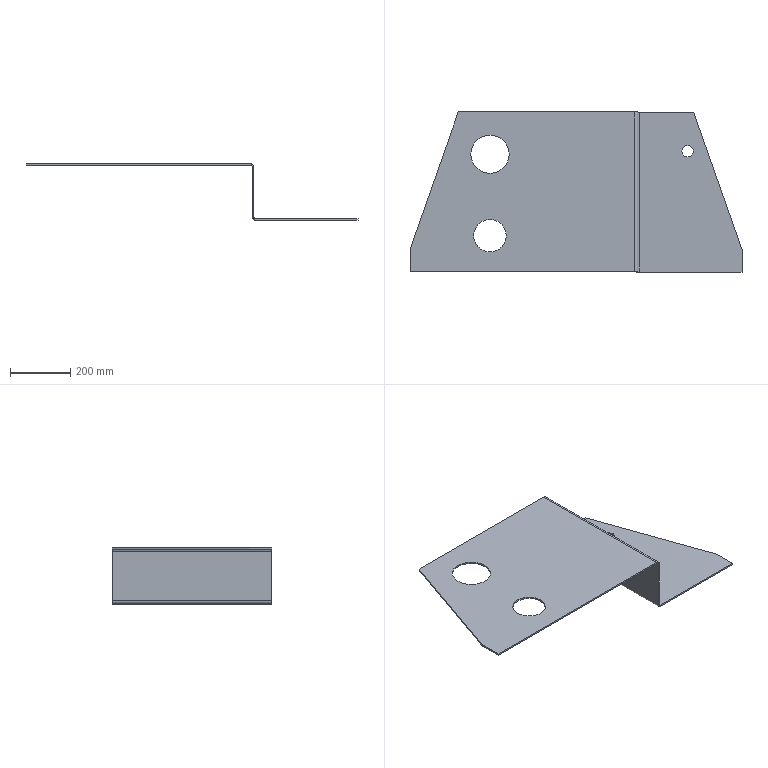Part | SolidWorks | features Cut 2, EdgeFlange 2, ICE 2, FlatPattern 1, SMBaseFlange 1, SheetMetal 1, UnFold 1 | 1 solid | 30 faces | box 1100 x 530 x 187 mm | volume 2899151 mm3 | plane 20 | cylinder 10 | commonest cylinder face diameters 12 x2 22 x2 38 x2 108 x2 127 x2
STEP:
#1=CARTESIAN_POINT('',(389.,400.,-182.));
#2=VERTEX_POINT('',#1);
#3=CARTESIAN_POINT('',(351.,400.,-182.));
#4=VERTEX_POINT('',#3);
#5=CARTESIAN_POINT('',(370.,400.,-182.));
#6=DIRECTION('',(0.,0.,-1.));
#7=DIRECTION('',(-1.,0.,0.));
#8=AXIS2_PLACEMENT_3D('',#5,#6,#7);
#9=CIRCLE('',#8,19.);
#10=EDGE_CURVE('',#2,#4,#9,.T.);
#11=ORIENTED_EDGE('',*,*,#10,.F.);
#12=CARTESIAN_POINT('',(389.,400.,-187.));
#13=VERTEX_POINT('',#12);
#14=CARTESIAN_POINT('',(389.,400.,-177.));
#15=DIRECTION('',(0.,0.,-1.));
#16=VECTOR('',#15,1000.);
#17=LINE('',#14,#16);
#18=EDGE_CURVE('',#2,#13,#17,.T.);
#19=ORIENTED_EDGE('',*,*,#18,.T.);
#20=CARTESIAN_POINT('',(351.,400.,-187.));
#21=VERTEX_POINT('',#20);
#22=CARTESIAN_POINT('',(370.,400.,-187.));
#23=DIRECTION('',(0.,0.,-1.));
#24=DIRECTION('',(-1.,0.,0.));
#25=AXIS2_PLACEMENT_3D('',#22,#23,#24);
#26=CIRCLE('',#25,19.);
#27=EDGE_CURVE('',#13,#21,#26,.T.);
#28=ORIENTED_EDGE('',*,*,#27,.T.);
#29=CARTESIAN_POINT('',(351.,400.,-177.));
#30=DIRECTION('',(0.,0.,-1.));
#31=VECTOR('',#30,1000.);
#32=LINE('',#29,#31);
#33=EDGE_CURVE('',#4,#21,#32,.T.);
#34=ORIENTED_EDGE('',*,*,#33,.F.);
#35=EDGE_LOOP('',(#11,#19,#28,#34));
#36=FACE_OUTER_BOUND('',#35,.T.);
#37=CARTESIAN_POINT('',(370.,400.,-177.));
#38=DIRECTION('',(0.,0.,-1.));
#39=DIRECTION('',(-1.,0.,0.));
#40=AXIS2_PLACEMENT_3D('',#37,#38,#39);
#41=CYLINDRICAL_SURFACE('',#40,19.);
#42=ADVANCED_FACE('',(#36),#41,.F.);
#43=CARTESIAN_POINT('',(-231.,120.,0.));
#44=VERTEX_POINT('',#43);
#45=CARTESIAN_POINT('',(-339.,120.,0.));
#46=VERTEX_POINT('',#45);
#47=CARTESIAN_POINT('',(-285.,120.,0.));
#48=DIRECTION('',(0.,0.,-1.));
#49=DIRECTION('',(-1.,0.,0.));
#50=AXIS2_PLACEMENT_3D('',#47,#48,#49);
#51=CIRCLE('',#50,54.);
#52=EDGE_CURVE('',#44,#46,#51,.T.);
#53=ORIENTED_EDGE('',*,*,#52,.F.);
#54=CARTESIAN_POINT('',(-231.,120.,-5.));
#55=VERTEX_POINT('',#54);
#56=CARTESIAN_POINT('',(-231.,120.,265.));
#57=DIRECTION('',(0.,0.,-1.));
#58=VECTOR('',#57,1000.);
#59=LINE('',#56,#58);
#60=EDGE_CURVE('',#44,#55,#59,.T.);
#61=ORIENTED_EDGE('',*,*,#60,.T.);
#62=CARTESIAN_POINT('',(-339.,120.,-5.));
#63=VERTEX_POINT('',#62);
#64=CARTESIAN_POINT('',(-285.,120.,-5.));
#65=DIRECTION('',(0.,0.,-1.));
#66=DIRECTION('',(-1.,0.,0.));
#67=AXIS2_PLACEMENT_3D('',#64,#65,#66);
#68=CIRCLE('',#67,54.);
#69=EDGE_CURVE('',#55,#63,#68,.T.);
#70=ORIENTED_EDGE('',*,*,#69,.T.);
#71=CARTESIAN_POINT('',(-339.,120.,265.));
#72=DIRECTION('',(0.,0.,-1.));
#73=VECTOR('',#72,1000.);
#74=LINE('',#71,#73);
#75=EDGE_CURVE('',#46,#63,#74,.T.);
#76=ORIENTED_EDGE('',*,*,#75,.F.);
#77=EDGE_LOOP('',(#53,#61,#70,#76));
#78=FACE_OUTER_BOUND('',#77,.T.);
#79=CARTESIAN_POINT('',(-285.,120.,265.));
#80=DIRECTION('',(0.,0.,-1.));
#81=DIRECTION('',(-1.,0.,0.));
#82=AXIS2_PLACEMENT_3D('',#79,#80,#81);
#83=CYLINDRICAL_SURFACE('',#82,54.);
#84=ADVANCED_FACE('',(#78),#83,.F.);
#85=CARTESIAN_POINT('',(-221.5,390.,0.));
#86=VERTEX_POINT('',#85);
#87=CARTESIAN_POINT('',(-348.5,390.,0.));
#88=VERTEX_POINT('',#87);
#89=CARTESIAN_POINT('',(-285.,390.,0.));
#90=DIRECTION('',(0.,0.,-1.));
#91=DIRECTION('',(-1.,0.,0.));
#92=AXIS2_PLACEMENT_3D('',#89,#90,#91);
#93=CIRCLE('',#92,63.5);
#94=EDGE_CURVE('',#86,#88,#93,.T.);
#95=ORIENTED_EDGE('',*,*,#94,.F.);
#96=CARTESIAN_POINT('',(-221.5,390.,-5.));
#97=VERTEX_POINT('',#96);
#98=CARTESIAN_POINT('',(-221.5,390.,265.));
#99=DIRECTION('',(0.,0.,-1.));
#100=VECTOR('',#99,1000.);
#101=LINE('',#98,#100);
#102=EDGE_CURVE('',#86,#97,#101,.T.);
#103=ORIENTED_EDGE('',*,*,#102,.T.);
#104=CARTESIAN_POINT('',(-348.5,390.,-5.));
#105=VERTEX_POINT('',#104);
#106=CARTESIAN_POINT('',(-285.,390.,-5.));
#107=DIRECTION('',(0.,0.,-1.));
#108=DIRECTION('',(-1.,0.,0.));
#109=AXIS2_PLACEMENT_3D('',#106,#107,#108);
#110=CIRCLE('',#109,63.5);
#111=EDGE_CURVE('',#97,#105,#110,.T.);
#112=ORIENTED_EDGE('',*,*,#111,.T.);
#113=CARTESIAN_POINT('',(-348.5,390.,265.));
#114=DIRECTION('',(0.,0.,-1.));
#115=VECTOR('',#114,1000.);
#116=LINE('',#113,#115);
#117=EDGE_CURVE('',#88,#105,#116,.T.);
#118=ORIENTED_EDGE('',*,*,#117,.F.);
#119=EDGE_LOOP('',(#95,#103,#112,#118));
#120=FACE_OUTER_BOUND('',#119,.T.);
#121=CARTESIAN_POINT('',(-285.,390.,265.));
#122=DIRECTION('',(0.,0.,-1.));
#123=DIRECTION('',(-1.,0.,0.));
#124=AXIS2_PLACEMENT_3D('',#121,#122,#123);
#125=CYLINDRICAL_SURFACE('',#124,63.5);
#126=ADVANCED_FACE('',(#120),#125,.F.);
#127=CARTESIAN_POINT('',(390.,530.,-182.));
#128=VERTEX_POINT('',#127);
#129=CARTESIAN_POINT('',(211.,530.,-182.));
#130=VERTEX_POINT('',#129);
#131=CARTESIAN_POINT('',(0.,530.,-182.));
#132=DIRECTION('',(-1.,0.,0.));
#133=VECTOR('',#132,1000.);
#134=LINE('',#131,#133);
#135=EDGE_CURVE('',#128,#130,#134,.T.);
#136=ORIENTED_EDGE('',*,*,#135,.F.);
#137=CARTESIAN_POINT('',(390.,530.,-187.));
#138=VERTEX_POINT('',#137);
#139=CARTESIAN_POINT('',(390.,530.,-187.));
#140=DIRECTION('',(0.,0.,1.));
#141=VECTOR('',#140,1000.);
#142=LINE('',#139,#141);
#143=EDGE_CURVE('',#138,#128,#142,.T.);
#144=ORIENTED_EDGE('',*,*,#143,.F.);
#145=CARTESIAN_POINT('',(211.,530.,-187.));
#146=VERTEX_POINT('',#145);
#147=CARTESIAN_POINT('',(205.,530.,-187.));
#148=DIRECTION('',(-1.,0.,0.));
#149=VECTOR('',#148,1000.);
#150=LINE('',#147,#149);
#151=EDGE_CURVE('',#138,#146,#150,.T.);
#152=ORIENTED_EDGE('',*,*,#151,.T.);
#153=CARTESIAN_POINT('',(211.,530.,-182.));
#154=DIRECTION('',(0.,0.,-1.));
#155=VECTOR('',#154,1000.);
#156=LINE('',#153,#155);
#157=EDGE_CURVE('',#130,#146,#156,.T.);
#158=ORIENTED_EDGE('',*,*,#157,.F.);
#159=EDGE_LOOP('',(#136,#144,#152,#158));
#160=FACE_OUTER_BOUND('',#159,.T.);
#161=CARTESIAN_POINT('',(205.,530.,-187.));
#162=DIRECTION('',(0.,1.,0.));
#163=DIRECTION('',(-1.,0.,0.));
#164=AXIS2_PLACEMENT_3D('',#161,#162,#163);
#165=PLANE('',#164);
#166=ADVANCED_FACE('',(#160),#165,.T.);
#167=CARTESIAN_POINT('',(370.,400.,-187.));
#168=DIRECTION('',(0.,0.,-1.));
#169=DIRECTION('',(-1.,0.,0.));
#170=AXIS2_PLACEMENT_3D('',#167,#168,#169);
#171=CIRCLE('',#170,19.);
#172=EDGE_CURVE('',#21,#13,#171,.T.);
#173=ORIENTED_EDGE('',*,*,#172,.F.);
#174=ORIENTED_EDGE('',*,*,#27,.F.);
#175=EDGE_LOOP('',(#173,#174));
#176=FACE_BOUND('',#175,.T.);
#177=ORIENTED_EDGE('',*,*,#151,.F.);
#178=CARTESIAN_POINT('',(550.,75.,-187.));
#179=VERTEX_POINT('',#178);
#180=CARTESIAN_POINT('',(512.945,180.376,-187.));
#181=DIRECTION('',(0.3317,-0.9434,0.));
#182=VECTOR('',#181,1000.);
#183=LINE('',#180,#182);
#184=EDGE_CURVE('',#138,#179,#183,.T.);
#185=ORIENTED_EDGE('',*,*,#184,.T.);
#186=CARTESIAN_POINT('',(550.,0.,-187.));
#187=VERTEX_POINT('',#186);
#188=CARTESIAN_POINT('',(550.,530.,-187.));
#189=DIRECTION('',(0.,1.,0.));
#190=VECTOR('',#189,1000.);
#191=LINE('',#188,#190);
#192=EDGE_CURVE('',#187,#179,#191,.T.);
#193=ORIENTED_EDGE('',*,*,#192,.F.);
#194=CARTESIAN_POINT('',(211.,0.,-187.));
#195=VERTEX_POINT('',#194);
#196=CARTESIAN_POINT('',(550.,0.,-187.));
#197=DIRECTION('',(1.,0.,0.));
#198=VECTOR('',#197,1000.);
#199=LINE('',#196,#198);
#200=EDGE_CURVE('',#195,#187,#199,.T.);
#201=ORIENTED_EDGE('',*,*,#200,.F.);
#202=CARTESIAN_POINT('',(211.,0.,-187.));
#203=DIRECTION('',(0.,1.,0.));
#204=VECTOR('',#203,1000.);
#205=LINE('',#202,#204);
#206=EDGE_CURVE('',#195,#146,#205,.T.);
#207=ORIENTED_EDGE('',*,*,#206,.T.);
#208=EDGE_LOOP('',(#177,#185,#193,#201,#207));
#209=FACE_OUTER_BOUND('',#208,.T.);
#210=CARTESIAN_POINT('',(0.,0.,-187.));
#211=DIRECTION('',(0.,0.,-1.));
#212=DIRECTION('',(-1.,0.,0.));
#213=AXIS2_PLACEMENT_3D('',#210,#211,#212);
#214=PLANE('',#213);
#215=ADVANCED_FACE('',(#176,#209),#214,.T.);
#216=CARTESIAN_POINT('',(370.,400.,-182.));
#217=DIRECTION('',(0.,0.,-1.));
#218=DIRECTION('',(-1.,0.,0.));
#219=AXIS2_PLACEMENT_3D('',#216,#217,#218);
#220=CIRCLE('',#219,19.);
#221=EDGE_CURVE('',#4,#2,#220,.T.);
#222=ORIENTED_EDGE('',*,*,#221,.T.);
#223=ORIENTED_EDGE('',*,*,#10,.T.);
#224=EDGE_LOOP('',(#222,#223));
#225=FACE_BOUND('',#224,.T.);
#226=CARTESIAN_POINT('',(550.,75.,-182.));
#227=VERTEX_POINT('',#226);
#228=CARTESIAN_POINT('',(512.945,180.376,-182.));
#229=DIRECTION('',(0.3317,-0.9434,0.));
#230=VECTOR('',#229,1000.);
#231=LINE('',#228,#230);
#232=EDGE_CURVE('',#128,#227,#231,.T.);
#233=ORIENTED_EDGE('',*,*,#232,.F.);
#234=ORIENTED_EDGE('',*,*,#135,.T.);
#235=CARTESIAN_POINT('',(211.,0.,-182.));
#236=VERTEX_POINT('',#235);
#237=CARTESIAN_POINT('',(211.,0.,-182.));
#238=DIRECTION('',(0.,1.,0.));
#239=VECTOR('',#238,1000.);
#240=LINE('',#237,#239);
#241=EDGE_CURVE('',#236,#130,#240,.T.);
#242=ORIENTED_EDGE('',*,*,#241,.F.);
#243=CARTESIAN_POINT('',(550.,0.,-182.));
#244=VERTEX_POINT('',#243);
#245=CARTESIAN_POINT('',(0.,0.,-182.));
#246=DIRECTION('',(1.,0.,0.));
#247=VECTOR('',#246,1000.);
#248=LINE('',#245,#247);
#249=EDGE_CURVE('',#236,#244,#248,.T.);
#250=ORIENTED_EDGE('',*,*,#249,.T.);
#251=CARTESIAN_POINT('',(550.,0.,-182.));
#252=DIRECTION('',(0.,1.,0.));
#253=VECTOR('',#252,1000.);
#254=LINE('',#251,#253);
#255=EDGE_CURVE('',#244,#227,#254,.T.);
#256=ORIENTED_EDGE('',*,*,#255,.T.);
#257=EDGE_LOOP('',(#233,#234,#242,#250,#256));
#258=FACE_OUTER_BOUND('',#257,.T.);
#259=CARTESIAN_POINT('',(0.,0.,-182.));
#260=DIRECTION('',(0.,0.,-1.));
#261=DIRECTION('',(-1.,0.,0.));
#262=AXIS2_PLACEMENT_3D('',#259,#260,#261);
#263=PLANE('',#262);
#264=ADVANCED_FACE('',(#225,#258),#263,.F.);
#265=ORIENTED_EDGE('',*,*,#192,.T.);
#266=CARTESIAN_POINT('',(550.,75.,-187.));
#267=DIRECTION('',(0.,0.,1.));
#268=VECTOR('',#267,1000.);
#269=LINE('',#266,#268);
#270=EDGE_CURVE('',#179,#227,#269,.T.);
#271=ORIENTED_EDGE('',*,*,#270,.T.);
#272=ORIENTED_EDGE('',*,*,#255,.F.);
#273=CARTESIAN_POINT('',(550.,0.,-187.));
#274=DIRECTION('',(0.,0.,1.));
#275=VECTOR('',#274,1000.);
#276=LINE('',#273,#275);
#277=EDGE_CURVE('',#187,#244,#276,.T.);
#278=ORIENTED_EDGE('',*,*,#277,.F.);
#279=EDGE_LOOP('',(#265,#271,#272,#278));
#280=FACE_OUTER_BOUND('',#279,.T.);
#281=CARTESIAN_POINT('',(550.,530.,-187.));
#282=DIRECTION('',(1.,0.,0.));
#283=DIRECTION('',(0.,1.,0.));
#284=AXIS2_PLACEMENT_3D('',#281,#282,#283);
#285=PLANE('',#284);
#286=ADVANCED_FACE('',(#280),#285,.T.);
#287=CARTESIAN_POINT('',(205.,530.,-11.));
#288=VERTEX_POINT('',#287);
#289=CARTESIAN_POINT('',(205.,530.,-176.));
#290=VERTEX_POINT('',#289);
#291=CARTESIAN_POINT('',(205.,530.,-187.));
#292=DIRECTION('',(0.,0.,-1.));
#293=VECTOR('',#292,1000.);
#294=LINE('',#291,#293);
#295=EDGE_CURVE('',#288,#290,#294,.T.);
#296=ORIENTED_EDGE('',*,*,#295,.T.);
#297=CARTESIAN_POINT('',(200.,530.,-176.));
#298=VERTEX_POINT('',#297);
#299=CARTESIAN_POINT('',(205.,530.,-176.));
#300=DIRECTION('',(-1.,0.,0.));
#301=VECTOR('',#300,1000.);
#302=LINE('',#299,#301);
#303=EDGE_CURVE('',#290,#298,#302,.T.);
#304=ORIENTED_EDGE('',*,*,#303,.T.);
#305=CARTESIAN_POINT('',(200.,530.,-11.));
#306=VERTEX_POINT('',#305);
#307=CARTESIAN_POINT('',(200.,530.,0.));
#308=DIRECTION('',(0.,0.,-1.));
#309=VECTOR('',#308,1000.);
#310=LINE('',#307,#309);
#311=EDGE_CURVE('',#306,#298,#310,.T.);
#312=ORIENTED_EDGE('',*,*,#311,.F.);
#313=CARTESIAN_POINT('',(205.,530.,-11.));
#314=DIRECTION('',(1.,0.,0.));
#315=VECTOR('',#314,1000.);
#316=LINE('',#313,#315);
#317=EDGE_CURVE('',#306,#288,#316,.T.);
#318=ORIENTED_EDGE('',*,*,#317,.T.);
#319=EDGE_LOOP('',(#296,#304,#312,#318));
#320=FACE_OUTER_BOUND('',#319,.T.);
#321=CARTESIAN_POINT('',(205.,530.,-187.));
#322=DIRECTION('',(0.,1.,0.));
#323=DIRECTION('',(-1.,0.,0.));
#324=AXIS2_PLACEMENT_3D('',#321,#322,#323);
#325=PLANE('',#324);
#326=ADVANCED_FACE('',(#320),#325,.T.);
#327=CARTESIAN_POINT('',(205.,0.,-176.));
#328=VERTEX_POINT('',#327);
#329=CARTESIAN_POINT('',(205.,0.,-11.));
#330=VERTEX_POINT('',#329);
#331=CARTESIAN_POINT('',(205.,0.,-5.));
#332=DIRECTION('',(0.,0.,1.));
#333=VECTOR('',#332,1000.);
#334=LINE('',#331,#333);
#335=EDGE_CURVE('',#328,#330,#334,.T.);
#336=ORIENTED_EDGE('',*,*,#335,.F.);
#337=CARTESIAN_POINT('',(205.,530.,-176.));
#338=DIRECTION('',(0.,-1.,0.));
#339=VECTOR('',#338,1000.);
#340=LINE('',#337,#339);
#341=EDGE_CURVE('',#290,#328,#340,.T.);
#342=ORIENTED_EDGE('',*,*,#341,.F.);
#343=ORIENTED_EDGE('',*,*,#295,.F.);
#344=CARTESIAN_POINT('',(205.,0.,-11.));
#345=DIRECTION('',(0.,-1.,0.));
#346=VECTOR('',#345,1000.);
#347=LINE('',#344,#346);
#348=EDGE_CURVE('',#288,#330,#347,.T.);
#349=ORIENTED_EDGE('',*,*,#348,.T.);
#350=EDGE_LOOP('',(#336,#342,#343,#349));
#351=FACE_OUTER_BOUND('',#350,.T.);
#352=CARTESIAN_POINT('',(205.,0.,0.));
#353=DIRECTION('',(1.,0.,0.));
#354=DIRECTION('',(0.,0.,-1.));
#355=AXIS2_PLACEMENT_3D('',#352,#353,#354);
#356=PLANE('',#355);
#357=ADVANCED_FACE('',(#351),#356,.T.);
#358=CARTESIAN_POINT('',(200.,0.,-176.));
#359=VERTEX_POINT('',#358);
#360=CARTESIAN_POINT('',(200.,530.,-176.));
#361=DIRECTION('',(0.,-1.,0.));
#362=VECTOR('',#361,1000.);
#363=LINE('',#360,#362);
#364=EDGE_CURVE('',#298,#359,#363,.T.);
#365=ORIENTED_EDGE('',*,*,#364,.T.);
#366=CARTESIAN_POINT('',(200.,0.,-11.));
#367=VERTEX_POINT('',#366);
#368=CARTESIAN_POINT('',(200.,0.,0.));
#369=DIRECTION('',(0.,0.,1.));
#370=VECTOR('',#369,1000.);
#371=LINE('',#368,#370);
#372=EDGE_CURVE('',#359,#367,#371,.T.);
#373=ORIENTED_EDGE('',*,*,#372,.T.);
#374=CARTESIAN_POINT('',(200.,530.,-11.));
#375=DIRECTION('',(0.,-1.,0.));
#376=VECTOR('',#375,1000.);
#377=LINE('',#374,#376);
#378=EDGE_CURVE('',#306,#367,#377,.T.);
#379=ORIENTED_EDGE('',*,*,#378,.F.);
#380=ORIENTED_EDGE('',*,*,#311,.T.);
#381=EDGE_LOOP('',(#365,#373,#379,#380));
#382=FACE_OUTER_BOUND('',#381,.T.);
#383=CARTESIAN_POINT('',(200.,0.,0.));
#384=DIRECTION('',(1.,0.,0.));
#385=DIRECTION('',(0.,0.,-1.));
#386=AXIS2_PLACEMENT_3D('',#383,#384,#385);
#387=PLANE('',#386);
#388=ADVANCED_FACE('',(#382),#387,.F.);
#389=CARTESIAN_POINT('',(-550.,0.,-5.));
#390=VERTEX_POINT('',#389);
#391=CARTESIAN_POINT('',(194.,0.,-5.));
#392=VERTEX_POINT('',#391);
#393=CARTESIAN_POINT('',(-550.,0.,-5.));
#394=DIRECTION('',(1.,0.,0.));
#395=VECTOR('',#394,1000.);
#396=LINE('',#393,#395);
#397=EDGE_CURVE('',#390,#392,#396,.T.);
#398=ORIENTED_EDGE('',*,*,#397,.T.);
#399=CARTESIAN_POINT('',(194.,0.,0.));
#400=VERTEX_POINT('',#399);
#401=CARTESIAN_POINT('',(194.,0.,-5.));
#402=DIRECTION('',(0.,0.,1.));
#403=VECTOR('',#402,1000.);
#404=LINE('',#401,#403);
#405=EDGE_CURVE('',#392,#400,#404,.T.);
#406=ORIENTED_EDGE('',*,*,#405,.T.);
#407=CARTESIAN_POINT('',(-550.,0.,0.));
#408=VERTEX_POINT('',#407);
#409=CARTESIAN_POINT('',(-550.,0.,0.));
#410=DIRECTION('',(1.,0.,0.));
#411=VECTOR('',#410,1000.);
#412=LINE('',#409,#411);
#413=EDGE_CURVE('',#408,#400,#412,.T.);
#414=ORIENTED_EDGE('',*,*,#413,.F.);
#415=CARTESIAN_POINT('',(-550.,0.,-5.));
#416=DIRECTION('',(0.,0.,1.));
#417=VECTOR('',#416,1000.);
#418=LINE('',#415,#417);
#419=EDGE_CURVE('',#390,#408,#418,.T.);
#420=ORIENTED_EDGE('',*,*,#419,.F.);
#421=EDGE_LOOP('',(#398,#406,#414,#420));
#422=FACE_OUTER_BOUND('',#421,.T.);
#423=CARTESIAN_POINT('',(-550.,0.,-5.));
#424=DIRECTION('',(0.,-1.,0.));
#425=DIRECTION('',(0.,0.,-1.));
#426=AXIS2_PLACEMENT_3D('',#423,#424,#425);
#427=PLANE('',#426);
#428=ADVANCED_FACE('',(#422),#427,.T.);
#429=CARTESIAN_POINT('',(-285.,120.,-5.));
#430=DIRECTION('',(0.,0.,-1.));
#431=DIRECTION('',(-1.,0.,0.));
#432=AXIS2_PLACEMENT_3D('',#429,#430,#431);
#433=CIRCLE('',#432,54.);
#434=EDGE_CURVE('',#63,#55,#433,.T.);
#435=ORIENTED_EDGE('',*,*,#434,.F.);
#436=ORIENTED_EDGE('',*,*,#69,.F.);
#437=EDGE_LOOP('',(#435,#436));
#438=FACE_BOUND('',#437,.T.);
#439=CARTESIAN_POINT('',(-285.,390.,-5.));
#440=DIRECTION('',(0.,0.,-1.));
#441=DIRECTION('',(-1.,0.,0.));
#442=AXIS2_PLACEMENT_3D('',#439,#440,#441);
#443=CIRCLE('',#442,63.5);
#444=EDGE_CURVE('',#105,#97,#443,.T.);
#445=ORIENTED_EDGE('',*,*,#444,.F.);
#446=ORIENTED_EDGE('',*,*,#111,.F.);
#447=EDGE_LOOP('',(#445,#446));
#448=FACE_BOUND('',#447,.T.);
#449=CARTESIAN_POINT('',(194.,530.,-5.));
#450=VERTEX_POINT('',#449);
#451=CARTESIAN_POINT('',(-390.,530.,-5.));
#452=VERTEX_POINT('',#451);
#453=CARTESIAN_POINT('',(-390.,530.,-5.));
#454=DIRECTION('',(-1.,0.,0.));
#455=VECTOR('',#454,1000.);
#456=LINE('',#453,#455);
#457=EDGE_CURVE('',#450,#452,#456,.T.);
#458=ORIENTED_EDGE('',*,*,#457,.F.);
#459=CARTESIAN_POINT('',(194.,0.,-5.));
#460=DIRECTION('',(0.,1.,0.));
#461=VECTOR('',#460,1000.);
#462=LINE('',#459,#461);
#463=EDGE_CURVE('',#392,#450,#462,.T.);
#464=ORIENTED_EDGE('',*,*,#463,.F.);
#465=ORIENTED_EDGE('',*,*,#397,.F.);
#466=CARTESIAN_POINT('',(-550.,75.,-5.));
#467=VERTEX_POINT('',#466);
#468=CARTESIAN_POINT('',(-550.,0.,-5.));
#469=DIRECTION('',(0.,-1.,0.));
#470=VECTOR('',#469,1000.);
#471=LINE('',#468,#470);
#472=EDGE_CURVE('',#467,#390,#471,.T.);
#473=ORIENTED_EDGE('',*,*,#472,.F.);
#474=CARTESIAN_POINT('',(-550.,75.,-5.));
#475=DIRECTION('',(-0.3317,-0.9434,0.));
#476=VECTOR('',#475,1000.);
#477=LINE('',#474,#476);
#478=EDGE_CURVE('',#452,#467,#477,.T.);
#479=ORIENTED_EDGE('',*,*,#478,.F.);
#480=EDGE_LOOP('',(#458,#464,#465,#473,#479));
#481=FACE_OUTER_BOUND('',#480,.T.);
#482=CARTESIAN_POINT('',(0.,0.,-5.));
#483=DIRECTION('',(0.,0.,-1.));
#484=DIRECTION('',(-1.,0.,0.));
#485=AXIS2_PLACEMENT_3D('',#482,#483,#484);
#486=PLANE('',#485);
#487=ADVANCED_FACE('',(#438,#448,#481),#486,.T.);
#488=CARTESIAN_POINT('',(-285.,120.,0.));
#489=DIRECTION('',(0.,0.,-1.));
#490=DIRECTION('',(-1.,0.,0.));
#491=AXIS2_PLACEMENT_3D('',#488,#489,#490);
#492=CIRCLE('',#491,54.);
#493=EDGE_CURVE('',#46,#44,#492,.T.);
#494=ORIENTED_EDGE('',*,*,#493,.T.);
#495=ORIENTED_EDGE('',*,*,#52,.T.);
#496=EDGE_LOOP('',(#494,#495));
#497=FACE_BOUND('',#496,.T.);
#498=CARTESIAN_POINT('',(-285.,390.,0.));
#499=DIRECTION('',(0.,0.,-1.));
#500=DIRECTION('',(-1.,0.,0.));
#501=AXIS2_PLACEMENT_3D('',#498,#499,#500);
#502=CIRCLE('',#501,63.5);
#503=EDGE_CURVE('',#88,#86,#502,.T.);
#504=ORIENTED_EDGE('',*,*,#503,.T.);
#505=ORIENTED_EDGE('',*,*,#94,.T.);
#506=EDGE_LOOP('',(#504,#505));
#507=FACE_BOUND('',#506,.T.);
#508=CARTESIAN_POINT('',(194.,530.,0.));
#509=VERTEX_POINT('',#508);
#510=CARTESIAN_POINT('',(194.,0.,0.));
#511=DIRECTION('',(0.,1.,0.));
#512=VECTOR('',#511,1000.);
#513=LINE('',#510,#512);
#514=EDGE_CURVE('',#400,#509,#513,.T.);
#515=ORIENTED_EDGE('',*,*,#514,.T.);
#516=CARTESIAN_POINT('',(-390.,530.,0.));
#517=VERTEX_POINT('',#516);
#518=CARTESIAN_POINT('',(-390.,530.,0.));
#519=DIRECTION('',(-1.,0.,0.));
#520=VECTOR('',#519,1000.);
#521=LINE('',#518,#520);
#522=EDGE_CURVE('',#509,#517,#521,.T.);
#523=ORIENTED_EDGE('',*,*,#522,.T.);
#524=CARTESIAN_POINT('',(-550.,75.,0.));
#525=VERTEX_POINT('',#524);
#526=CARTESIAN_POINT('',(-550.,75.,0.));
#527=DIRECTION('',(-0.3317,-0.9434,0.));
#528=VECTOR('',#527,1000.);
#529=LINE('',#526,#528);
#530=EDGE_CURVE('',#517,#525,#529,.T.);
#531=ORIENTED_EDGE('',*,*,#530,.T.);
#532=CARTESIAN_POINT('',(-550.,0.,0.));
#533=DIRECTION('',(0.,-1.,0.));
#534=VECTOR('',#533,1000.);
#535=LINE('',#532,#534);
#536=EDGE_CURVE('',#525,#408,#535,.T.);
#537=ORIENTED_EDGE('',*,*,#536,.T.);
#538=ORIENTED_EDGE('',*,*,#413,.T.);
#539=EDGE_LOOP('',(#515,#523,#531,#537,#538));
#540=FACE_OUTER_BOUND('',#539,.T.);
#541=CARTESIAN_POINT('',(0.,0.,0.));
#542=DIRECTION('',(0.,0.,-1.));
#543=DIRECTION('',(-1.,0.,0.));
#544=AXIS2_PLACEMENT_3D('',#541,#542,#543);
#545=PLANE('',#544);
#546=ADVANCED_FACE('',(#497,#507,#540),#545,.F.);
#547=CARTESIAN_POINT('',(194.,530.,-5.));
#548=DIRECTION('',(0.,0.,1.));
#549=VECTOR('',#548,1000.);
#550=LINE('',#547,#549);
#551=EDGE_CURVE('',#450,#509,#550,.T.);
#552=ORIENTED_EDGE('',*,*,#551,.F.);
#553=ORIENTED_EDGE('',*,*,#457,.T.);
#554=CARTESIAN_POINT('',(-390.,530.,-5.));
#555=DIRECTION('',(0.,0.,1.));
#556=VECTOR('',#555,1000.);
#557=LINE('',#554,#556);
#558=EDGE_CURVE('',#452,#517,#557,.T.);
#559=ORIENTED_EDGE('',*,*,#558,.T.);
#560=ORIENTED_EDGE('',*,*,#522,.F.);
#561=EDGE_LOOP('',(#552,#553,#559,#560));
#562=FACE_OUTER_BOUND('',#561,.T.);
#563=CARTESIAN_POINT('',(-390.,530.,-5.));
#564=DIRECTION('',(0.,1.,0.));
#565=DIRECTION('',(0.,0.,1.));
#566=AXIS2_PLACEMENT_3D('',#563,#564,#565);
#567=PLANE('',#566);
#568=ADVANCED_FACE('',(#562),#567,.T.);
#569=ORIENTED_EDGE('',*,*,#536,.F.);
#570=CARTESIAN_POINT('',(-550.,75.,-5.));
#571=DIRECTION('',(0.,0.,1.));
#572=VECTOR('',#571,1000.);
#573=LINE('',#570,#572);
#574=EDGE_CURVE('',#467,#525,#573,.T.);
#575=ORIENTED_EDGE('',*,*,#574,.F.);
#576=ORIENTED_EDGE('',*,*,#472,.T.);
#577=ORIENTED_EDGE('',*,*,#419,.T.);
#578=EDGE_LOOP('',(#569,#575,#576,#577));
#579=FACE_OUTER_BOUND('',#578,.T.);
#580=CARTESIAN_POINT('',(-550.,0.,-5.));
#581=DIRECTION('',(-1.,0.,0.));
#582=DIRECTION('',(0.,0.,1.));
#583=AXIS2_PLACEMENT_3D('',#580,#581,#582);
#584=PLANE('',#583);
#585=ADVANCED_FACE('',(#579),#584,.T.);
#586=ORIENTED_EDGE('',*,*,#530,.F.);
#587=ORIENTED_EDGE('',*,*,#558,.F.);
#588=ORIENTED_EDGE('',*,*,#478,.T.);
#589=ORIENTED_EDGE('',*,*,#574,.T.);
#590=EDGE_LOOP('',(#586,#587,#588,#589));
#591=FACE_OUTER_BOUND('',#590,.T.);
#592=CARTESIAN_POINT('',(-550.,75.,-5.));
#593=DIRECTION('',(-0.9434,0.3317,0.));
#594=DIRECTION('',(-0.3317,-0.9434,0.));
#595=AXIS2_PLACEMENT_3D('',#592,#593,#594);
#596=PLANE('',#595);
#597=ADVANCED_FACE('',(#591),#596,.T.);
#598=ORIENTED_EDGE('',*,*,#317,.F.);
#599=CARTESIAN_POINT('',(194.,530.,-11.));
#600=DIRECTION('',(0.,1.,0.));
#601=DIRECTION('',(0.,0.,-1.));
#602=AXIS2_PLACEMENT_3D('',#599,#600,#601);
#603=CIRCLE('',#602,6.);
#604=EDGE_CURVE('',#450,#306,#603,.T.);
#605=ORIENTED_EDGE('',*,*,#604,.F.);
#606=ORIENTED_EDGE('',*,*,#551,.T.);
#607=CARTESIAN_POINT('',(194.,530.,-11.));
#608=DIRECTION('',(0.,1.,0.));
#609=DIRECTION('',(0.,0.,-1.));
#610=AXIS2_PLACEMENT_3D('',#607,#608,#609);
#611=CIRCLE('',#610,11.);
#612=EDGE_CURVE('',#509,#288,#611,.T.);
#613=ORIENTED_EDGE('',*,*,#612,.T.);
#614=EDGE_LOOP('',(#598,#605,#606,#613));
#615=FACE_OUTER_BOUND('',#614,.T.);
#616=CARTESIAN_POINT('',(194.,530.,-11.));
#617=DIRECTION('',(0.,1.,0.));
#618=DIRECTION('',(0.,0.,1.));
#619=AXIS2_PLACEMENT_3D('',#616,#617,#618);
#620=PLANE('',#619);
#621=ADVANCED_FACE('',(#615),#620,.T.);
#622=CARTESIAN_POINT('',(194.,0.,-11.));
#623=DIRECTION('',(0.,-1.,0.));
#624=DIRECTION('',(0.,0.,-1.));
#625=AXIS2_PLACEMENT_3D('',#622,#623,#624);
#626=CIRCLE('',#625,6.);
#627=EDGE_CURVE('',#367,#392,#626,.T.);
#628=ORIENTED_EDGE('',*,*,#627,.F.);
#629=CARTESIAN_POINT('',(200.,0.,-11.));
#630=DIRECTION('',(1.,0.,0.));
#631=VECTOR('',#630,1000.);
#632=LINE('',#629,#631);
#633=EDGE_CURVE('',#367,#330,#632,.T.);
#634=ORIENTED_EDGE('',*,*,#633,.T.);
#635=CARTESIAN_POINT('',(194.,0.,-11.));
#636=DIRECTION('',(0.,-1.,0.));
#637=DIRECTION('',(0.,0.,-1.));
#638=AXIS2_PLACEMENT_3D('',#635,#636,#637);
#639=CIRCLE('',#638,11.);
#640=EDGE_CURVE('',#330,#400,#639,.T.);
#641=ORIENTED_EDGE('',*,*,#640,.T.);
#642=ORIENTED_EDGE('',*,*,#405,.F.);
#643=EDGE_LOOP('',(#628,#634,#641,#642));
#644=FACE_OUTER_BOUND('',#643,.T.);
#645=CARTESIAN_POINT('',(194.,0.,-11.));
#646=DIRECTION('',(0.,1.,0.));
#647=DIRECTION('',(0.,0.,1.));
#648=AXIS2_PLACEMENT_3D('',#645,#646,#647);
#649=PLANE('',#648);
#650=ADVANCED_FACE('',(#644),#649,.F.);
#651=ORIENTED_EDGE('',*,*,#514,.F.);
#652=ORIENTED_EDGE('',*,*,#640,.F.);
#653=ORIENTED_EDGE('',*,*,#348,.F.);
#654=ORIENTED_EDGE('',*,*,#612,.F.);
#655=EDGE_LOOP('',(#651,#652,#653,#654));
#656=FACE_OUTER_BOUND('',#655,.T.);
#657=CARTESIAN_POINT('',(194.,0.,-11.));
#658=DIRECTION('',(0.,-1.,0.));
#659=DIRECTION('',(1.,0.,0.));
#660=AXIS2_PLACEMENT_3D('',#657,#658,#659);
#661=CYLINDRICAL_SURFACE('',#660,11.);
#662=ADVANCED_FACE('',(#656),#661,.T.);
#663=ORIENTED_EDGE('',*,*,#463,.T.);
#664=ORIENTED_EDGE('',*,*,#604,.T.);
#665=ORIENTED_EDGE('',*,*,#378,.T.);
#666=ORIENTED_EDGE('',*,*,#627,.T.);
#667=EDGE_LOOP('',(#663,#664,#665,#666));
#668=FACE_OUTER_BOUND('',#667,.T.);
#669=CARTESIAN_POINT('',(194.,0.,-11.));
#670=DIRECTION('',(0.,-1.,0.));
#671=DIRECTION('',(1.,0.,0.));
#672=AXIS2_PLACEMENT_3D('',#669,#670,#671);
#673=CYLINDRICAL_SURFACE('',#672,6.);
#674=ADVANCED_FACE('',(#668),#673,.F.);
#675=CARTESIAN_POINT('',(205.,0.,-176.));
#676=DIRECTION('',(-1.,0.,0.));
#677=VECTOR('',#676,1000.);
#678=LINE('',#675,#677);
#679=EDGE_CURVE('',#328,#359,#678,.T.);
#680=ORIENTED_EDGE('',*,*,#679,.F.);
#681=ORIENTED_EDGE('',*,*,#335,.T.);
#682=ORIENTED_EDGE('',*,*,#633,.F.);
#683=ORIENTED_EDGE('',*,*,#372,.F.);
#684=EDGE_LOOP('',(#680,#681,#682,#683));
#685=FACE_OUTER_BOUND('',#684,.T.);
#686=CARTESIAN_POINT('',(205.,0.,-5.));
#687=DIRECTION('',(0.,-1.,0.));
#688=DIRECTION('',(1.,0.,0.));
#689=AXIS2_PLACEMENT_3D('',#686,#687,#688);
#690=PLANE('',#689);
#691=ADVANCED_FACE('',(#685),#690,.T.);
#692=CARTESIAN_POINT('',(211.,0.,-187.));
#693=DIRECTION('',(0.,0.,-1.));
#694=VECTOR('',#693,1000.);
#695=LINE('',#692,#694);
#696=EDGE_CURVE('',#236,#195,#695,.T.);
#697=ORIENTED_EDGE('',*,*,#696,.F.);
#698=CARTESIAN_POINT('',(211.,0.,-176.));
#699=DIRECTION('',(0.,-1.,0.));
#700=DIRECTION('',(0.,0.,1.));
#701=AXIS2_PLACEMENT_3D('',#698,#699,#700);
#702=CIRCLE('',#701,6.);
#703=EDGE_CURVE('',#328,#236,#702,.T.);
#704=ORIENTED_EDGE('',*,*,#703,.F.);
#705=ORIENTED_EDGE('',*,*,#679,.T.);
#706=CARTESIAN_POINT('',(211.,0.,-176.));
#707=DIRECTION('',(0.,-1.,0.));
#708=DIRECTION('',(0.,0.,1.));
#709=AXIS2_PLACEMENT_3D('',#706,#707,#708);
#710=CIRCLE('',#709,11.);
#711=EDGE_CURVE('',#359,#195,#710,.T.);
#712=ORIENTED_EDGE('',*,*,#711,.T.);
#713=EDGE_LOOP('',(#697,#704,#705,#712));
#714=FACE_OUTER_BOUND('',#713,.T.);
#715=CARTESIAN_POINT('',(211.,0.,-176.));
#716=DIRECTION('',(0.,-1.,0.));
#717=DIRECTION('',(0.,0.,-1.));
#718=AXIS2_PLACEMENT_3D('',#715,#716,#717);
#719=PLANE('',#718);
#720=ADVANCED_FACE('',(#714),#719,.T.);
#721=CARTESIAN_POINT('',(211.,530.,-176.));
#722=DIRECTION('',(0.,1.,0.));
#723=DIRECTION('',(0.,0.,1.));
#724=AXIS2_PLACEMENT_3D('',#721,#722,#723);
#725=CIRCLE('',#724,6.);
#726=EDGE_CURVE('',#130,#290,#725,.T.);
#727=ORIENTED_EDGE('',*,*,#726,.F.);
#728=ORIENTED_EDGE('',*,*,#157,.T.);
#729=CARTESIAN_POINT('',(211.,530.,-176.));
#730=DIRECTION('',(0.,1.,0.));
#731=DIRECTION('',(0.,0.,1.));
#732=AXIS2_PLACEMENT_3D('',#729,#730,#731);
#733=CIRCLE('',#732,11.);
#734=EDGE_CURVE('',#146,#298,#733,.T.);
#735=ORIENTED_EDGE('',*,*,#734,.T.);
#736=ORIENTED_EDGE('',*,*,#303,.F.);
#737=EDGE_LOOP('',(#727,#728,#735,#736));
#738=FACE_OUTER_BOUND('',#737,.T.);
#739=CARTESIAN_POINT('',(211.,530.,-176.));
#740=DIRECTION('',(0.,-1.,0.));
#741=DIRECTION('',(0.,0.,-1.));
#742=AXIS2_PLACEMENT_3D('',#739,#740,#741);
#743=PLANE('',#742);
#744=ADVANCED_FACE('',(#738),#743,.F.);
#745=ORIENTED_EDGE('',*,*,#364,.F.);
#746=ORIENTED_EDGE('',*,*,#734,.F.);
#747=ORIENTED_EDGE('',*,*,#206,.F.);
#748=ORIENTED_EDGE('',*,*,#711,.F.);
#749=EDGE_LOOP('',(#745,#746,#747,#748));
#750=FACE_OUTER_BOUND('',#749,.T.);
#751=CARTESIAN_POINT('',(211.,530.,-176.));
#752=DIRECTION('',(0.,1.,0.));
#753=DIRECTION('',(0.,0.,-1.));
#754=AXIS2_PLACEMENT_3D('',#751,#752,#753);
#755=CYLINDRICAL_SURFACE('',#754,11.);
#756=ADVANCED_FACE('',(#750),#755,.T.);
#757=ORIENTED_EDGE('',*,*,#341,.T.);
#758=ORIENTED_EDGE('',*,*,#703,.T.);
#759=ORIENTED_EDGE('',*,*,#241,.T.);
#760=ORIENTED_EDGE('',*,*,#726,.T.);
#761=EDGE_LOOP('',(#757,#758,#759,#760));
#762=FACE_OUTER_BOUND('',#761,.T.);
#763=CARTESIAN_POINT('',(211.,530.,-176.));
#764=DIRECTION('',(0.,1.,0.));
#765=DIRECTION('',(0.,0.,-1.));
#766=AXIS2_PLACEMENT_3D('',#763,#764,#765);
#767=CYLINDRICAL_SURFACE('',#766,6.);
#768=ADVANCED_FACE('',(#762),#767,.F.);
#769=ORIENTED_EDGE('',*,*,#249,.F.);
#770=ORIENTED_EDGE('',*,*,#696,.T.);
#771=ORIENTED_EDGE('',*,*,#200,.T.);
#772=ORIENTED_EDGE('',*,*,#277,.T.);
#773=EDGE_LOOP('',(#769,#770,#771,#772));
#774=FACE_OUTER_BOUND('',#773,.T.);
#775=CARTESIAN_POINT('',(550.,0.,-187.));
#776=DIRECTION('',(0.,-1.,0.));
#777=DIRECTION('',(1.,0.,0.));
#778=AXIS2_PLACEMENT_3D('',#775,#776,#777);
#779=PLANE('',#778);
#780=ADVANCED_FACE('',(#774),#779,.T.);
#781=ORIENTED_EDGE('',*,*,#270,.F.);
#782=ORIENTED_EDGE('',*,*,#184,.F.);
#783=ORIENTED_EDGE('',*,*,#143,.T.);
#784=ORIENTED_EDGE('',*,*,#232,.T.);
#785=EDGE_LOOP('',(#781,#782,#783,#784));
#786=FACE_OUTER_BOUND('',#785,.T.);
#787=CARTESIAN_POINT('',(512.945,180.376,-187.));
#788=DIRECTION('',(0.9434,0.3317,0.));
#789=DIRECTION('',(0.3317,-0.9434,0.));
#790=AXIS2_PLACEMENT_3D('',#787,#788,#789);
#791=PLANE('',#790);
#792=ADVANCED_FACE('',(#786),#791,.T.);
#793=ORIENTED_EDGE('',*,*,#102,.F.);
#794=ORIENTED_EDGE('',*,*,#503,.F.);
#795=ORIENTED_EDGE('',*,*,#117,.T.);
#796=ORIENTED_EDGE('',*,*,#444,.T.);
#797=EDGE_LOOP('',(#793,#794,#795,#796));
#798=FACE_OUTER_BOUND('',#797,.T.);
#799=CARTESIAN_POINT('',(-285.,390.,265.));
#800=DIRECTION('',(0.,0.,-1.));
#801=DIRECTION('',(-1.,0.,0.));
#802=AXIS2_PLACEMENT_3D('',#799,#800,#801);
#803=CYLINDRICAL_SURFACE('',#802,63.5);
#804=ADVANCED_FACE('',(#798),#803,.F.);
#805=ORIENTED_EDGE('',*,*,#60,.F.);
#806=ORIENTED_EDGE('',*,*,#493,.F.);
#807=ORIENTED_EDGE('',*,*,#75,.T.);
#808=ORIENTED_EDGE('',*,*,#434,.T.);
#809=EDGE_LOOP('',(#805,#806,#807,#808));
#810=FACE_OUTER_BOUND('',#809,.T.);
#811=CARTESIAN_POINT('',(-285.,120.,265.));
#812=DIRECTION('',(0.,0.,-1.));
#813=DIRECTION('',(-1.,0.,0.));
#814=AXIS2_PLACEMENT_3D('',#811,#812,#813);
#815=CYLINDRICAL_SURFACE('',#814,54.);
#816=ADVANCED_FACE('',(#810),#815,.F.);
#817=ORIENTED_EDGE('',*,*,#18,.F.);
#818=ORIENTED_EDGE('',*,*,#221,.F.);
#819=ORIENTED_EDGE('',*,*,#33,.T.);
#820=ORIENTED_EDGE('',*,*,#172,.T.);
#821=EDGE_LOOP('',(#817,#818,#819,#820));
#822=FACE_OUTER_BOUND('',#821,.T.);
#823=CARTESIAN_POINT('',(370.,400.,-177.));
#824=DIRECTION('',(0.,0.,-1.));
#825=DIRECTION('',(-1.,0.,0.));
#826=AXIS2_PLACEMENT_3D('',#823,#824,#825);
#827=CYLINDRICAL_SURFACE('',#826,19.);
#828=ADVANCED_FACE('',(#822),#827,.F.);
#829=CLOSED_SHELL('',(#42,#84,#126,#166,#215,#264,#286,#326,#357,#388,#428,#487,#546,#568,#585,#597,#621,#650,#662,#674,#691,#720,#744,#756,#768,#780,#792,#804,#816,#828));
#830=MANIFOLD_SOLID_BREP('',#829);
#831=CARTESIAN_POINT('',(0.,0.,0.));
#832=DIRECTION('',(0.,0.,1.));
#833=DIRECTION('',(1.,0.,0.));
#834=AXIS2_PLACEMENT_3D('',#831,#832,#833);
#835=(LENGTH_UNIT()NAMED_UNIT(*)SI_UNIT(.MILLI.,.METRE.));
#836=UNCERTAINTY_MEASURE_WITH_UNIT(LENGTH_MEASURE(0.00001),#835,'','');
#837=(NAMED_UNIT(*)PLANE_ANGLE_UNIT()SI_UNIT($,.RADIAN.));
#838=(NAMED_UNIT(*)SI_UNIT($,.STERADIAN.)SOLID_ANGLE_UNIT());
#839=(GEOMETRIC_REPRESENTATION_CONTEXT(3)GLOBAL_UNCERTAINTY_ASSIGNED_CONTEXT((#836))GLOBAL_UNIT_ASSIGNED_CONTEXT((#835,#837,#838))REPRESENTATION_CONTEXT('',''));
#840=ADVANCED_BREP_SHAPE_REPRESENTATION('',(#830,#834),#839);